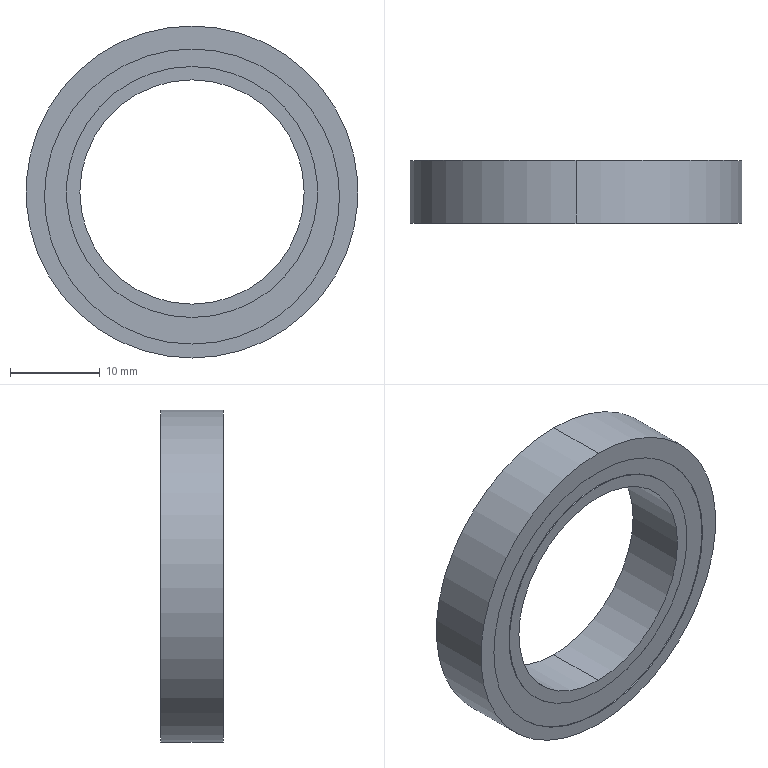Part | STEP file | Wheel bearing | 1 solid | 18 faces | box 37 x 7 x 37 mm | volume 4043 mm3 | cylinder 12 | plane 6 | commonest cylinder face diameters 27.974 x4 32.885 x4 25 x2 37 x2
STEP:
#1=CARTESIAN_POINT('',(0.,0.,0.));
#2=DIRECTION('',(0.,0.,1.));
#3=DIRECTION('',(1.,0.,0.));
#4=AXIS2_PLACEMENT_3D('',#1,#2,#3);
#5=CARTESIAN_POINT('',(0.,-3.4,13.987));
#6=VERTEX_POINT('',#5);
#7=CARTESIAN_POINT('',(0.,-3.4,-13.987));
#8=VERTEX_POINT('',#7);
#9=CARTESIAN_POINT('',(0.,-3.4,0.));
#10=DIRECTION('',(0.,1.,0.));
#11=DIRECTION('',(0.,0.,1.));
#12=AXIS2_PLACEMENT_3D('',#9,#10,#11);
#13=CIRCLE('',#12,13.987);
#14=CARTESIAN_POINT('',(0.,-3.4,0.));
#15=DIRECTION('',(0.,-1.,0.));
#16=DIRECTION('',(0.,0.,-1.));
#17=AXIS2_PLACEMENT_3D('',#14,#15,#16);
#18=CYLINDRICAL_SURFACE('',#17,13.987);
#19=CARTESIAN_POINT('',(3.142,0.));
#20=DIRECTION('',(-1.,0.));
#21=VECTOR('',#20,1.);
#22=LINE('',#19,#21);
#23=(GEOMETRIC_REPRESENTATION_CONTEXT(2)PARAMETRIC_REPRESENTATION_CONTEXT()REPRESENTATION_CONTEXT('',''));
#24=DEFINITIONAL_REPRESENTATION('',(#22),#23);
#25=PCURVE('',#18,#24);
#26=CARTESIAN_POINT('',(0.,-3.4,-0.506));
#27=DIRECTION('',(0.,-1.,0.));
#28=DIRECTION('',(0.,0.,1.));
#29=AXIS2_PLACEMENT_3D('',#26,#27,#28);
#30=PLANE('',#29);
#31=CARTESIAN_POINT('',(14.493,0.));
#32=CARTESIAN_POINT('',(14.493,-24.226));
#33=CARTESIAN_POINT('',(-6.487,-12.113));
#34=CARTESIAN_POINT('',(-27.468,0.));
#35=CARTESIAN_POINT('',(-6.487,12.113));
#36=CARTESIAN_POINT('',(14.493,24.226));
#37=CARTESIAN_POINT('',(14.493,0.));
#38=(BOUNDED_CURVE()B_SPLINE_CURVE(2,(#31,#32,#33,#34,#35,#36,#37),.UNSPECIFIED.,.T.,.F.)B_SPLINE_CURVE_WITH_KNOTS((1,2,2,2,2,1),(-2.094,0.,2.094,4.189,6.283,8.378),.UNSPECIFIED.)CURVE()GEOMETRIC_REPRESENTATION_ITEM()RATIONAL_B_SPLINE_CURVE((1.,0.5,1.,0.5,1.,0.5,1.))REPRESENTATION_ITEM(''));
#39=(GEOMETRIC_REPRESENTATION_CONTEXT(2)PARAMETRIC_REPRESENTATION_CONTEXT()REPRESENTATION_CONTEXT('',''));
#40=DEFINITIONAL_REPRESENTATION('',(#38),#39);
#41=PCURVE('',#30,#40);
#42=SURFACE_CURVE('',#13,(#25,#41),.PCURVE_S1.);
#43=EDGE_CURVE('',#6,#8,#42,.T.);
#44=ORIENTED_EDGE('',*,*,#43,.F.);
#45=CARTESIAN_POINT('',(0.,-3.5,13.987));
#46=VERTEX_POINT('',#45);
#47=CARTESIAN_POINT('',(0.,-3.4,13.987));
#48=DIRECTION('',(0.,-1.,0.));
#49=VECTOR('',#48,1.);
#50=LINE('',#47,#49);
#51=CARTESIAN_POINT('',(3.142,0.));
#52=DIRECTION('',(0.,1.));
#53=VECTOR('',#52,1.);
#54=LINE('',#51,#53);
#55=(GEOMETRIC_REPRESENTATION_CONTEXT(2)PARAMETRIC_REPRESENTATION_CONTEXT()REPRESENTATION_CONTEXT('',''));
#56=DEFINITIONAL_REPRESENTATION('',(#54),#55);
#57=PCURVE('',#18,#56);
#58=CARTESIAN_POINT('',(0.,-3.4,0.));
#59=DIRECTION('',(0.,-1.,0.));
#60=DIRECTION('',(0.,0.,-1.));
#61=AXIS2_PLACEMENT_3D('',#58,#59,#60);
#62=CYLINDRICAL_SURFACE('',#61,13.987);
#63=CARTESIAN_POINT('',(3.142,0.));
#64=DIRECTION('',(0.,1.));
#65=VECTOR('',#64,1.);
#66=LINE('',#63,#65);
#67=(GEOMETRIC_REPRESENTATION_CONTEXT(2)PARAMETRIC_REPRESENTATION_CONTEXT()REPRESENTATION_CONTEXT('',''));
#68=DEFINITIONAL_REPRESENTATION('',(#66),#67);
#69=PCURVE('',#62,#68);
#70=SURFACE_CURVE('',#50,(#57,#69),.PCURVE_S1.);
#71=EDGE_CURVE('',#6,#46,#70,.T.);
#72=ORIENTED_EDGE('',*,*,#71,.T.);
#73=CARTESIAN_POINT('',(0.,-3.5,-13.987));
#74=VERTEX_POINT('',#73);
#75=CARTESIAN_POINT('',(0.,-3.5,0.));
#76=DIRECTION('',(0.,1.,0.));
#77=DIRECTION('',(0.,0.,1.));
#78=AXIS2_PLACEMENT_3D('',#75,#76,#77);
#79=CIRCLE('',#78,13.987);
#80=CARTESIAN_POINT('',(3.142,0.1));
#81=DIRECTION('',(-1.,0.));
#82=VECTOR('',#81,1.);
#83=LINE('',#80,#82);
#84=(GEOMETRIC_REPRESENTATION_CONTEXT(2)PARAMETRIC_REPRESENTATION_CONTEXT()REPRESENTATION_CONTEXT('',''));
#85=DEFINITIONAL_REPRESENTATION('',(#83),#84);
#86=PCURVE('',#18,#85);
#87=CARTESIAN_POINT('',(0.,-3.5,0.));
#88=DIRECTION('',(0.,1.,0.));
#89=DIRECTION('',(0.,0.,1.));
#90=AXIS2_PLACEMENT_3D('',#87,#88,#89);
#91=PLANE('',#90);
#92=CARTESIAN_POINT('',(0.,0.));
#93=DIRECTION('',(1.,0.));
#94=AXIS2_PLACEMENT_2D('',#92,#93);
#95=CIRCLE('',#94,13.987);
#96=(GEOMETRIC_REPRESENTATION_CONTEXT(2)PARAMETRIC_REPRESENTATION_CONTEXT()REPRESENTATION_CONTEXT('',''));
#97=DEFINITIONAL_REPRESENTATION('',(#95),#96);
#98=PCURVE('',#91,#97);
#99=SURFACE_CURVE('',#79,(#86,#98),.PCURVE_S1.);
#100=EDGE_CURVE('',#46,#74,#99,.T.);
#101=ORIENTED_EDGE('',*,*,#100,.T.);
#102=CARTESIAN_POINT('',(0.,-3.4,-13.987));
#103=DIRECTION('',(0.,-1.,0.));
#104=VECTOR('',#103,1.);
#105=LINE('',#102,#104);
#106=CARTESIAN_POINT('',(0.,0.));
#107=DIRECTION('',(0.,1.));
#108=VECTOR('',#107,1.);
#109=LINE('',#106,#108);
#110=(GEOMETRIC_REPRESENTATION_CONTEXT(2)PARAMETRIC_REPRESENTATION_CONTEXT()REPRESENTATION_CONTEXT('',''));
#111=DEFINITIONAL_REPRESENTATION('',(#109),#110);
#112=PCURVE('',#18,#111);
#113=CARTESIAN_POINT('',(6.283,0.));
#114=DIRECTION('',(0.,1.));
#115=VECTOR('',#114,1.);
#116=LINE('',#113,#115);
#117=(GEOMETRIC_REPRESENTATION_CONTEXT(2)PARAMETRIC_REPRESENTATION_CONTEXT()REPRESENTATION_CONTEXT('',''));
#118=DEFINITIONAL_REPRESENTATION('',(#116),#117);
#119=PCURVE('',#62,#118);
#120=SURFACE_CURVE('',#105,(#112,#119),.PCURVE_S1.);
#121=EDGE_CURVE('',#8,#74,#120,.T.);
#122=ORIENTED_EDGE('',*,*,#121,.F.);
#123=EDGE_LOOP('',(#44,#72,#101,#122));
#124=FACE_BOUND('',#123,.T.);
#125=ADVANCED_FACE('',(#124),#18,.T.);
#126=CARTESIAN_POINT('',(0.,-3.4,-16.948));
#127=VERTEX_POINT('',#126);
#128=CARTESIAN_POINT('',(0.,-3.5,-16.948));
#129=VERTEX_POINT('',#128);
#130=CARTESIAN_POINT('',(0.,-3.4,-16.948));
#131=DIRECTION('',(0.,-1.,0.));
#132=VECTOR('',#131,1.);
#133=LINE('',#130,#132);
#134=CARTESIAN_POINT('',(0.,-3.4,-0.506));
#135=DIRECTION('',(0.,-1.,0.));
#136=DIRECTION('',(0.,0.,-1.));
#137=AXIS2_PLACEMENT_3D('',#134,#135,#136);
#138=CYLINDRICAL_SURFACE('',#137,16.442);
#139=CARTESIAN_POINT('',(6.283,0.));
#140=DIRECTION('',(0.,1.));
#141=VECTOR('',#140,1.);
#142=LINE('',#139,#141);
#143=(GEOMETRIC_REPRESENTATION_CONTEXT(2)PARAMETRIC_REPRESENTATION_CONTEXT()REPRESENTATION_CONTEXT('',''));
#144=DEFINITIONAL_REPRESENTATION('',(#142),#143);
#145=PCURVE('',#138,#144);
#146=CARTESIAN_POINT('',(0.,-3.4,-0.506));
#147=DIRECTION('',(0.,-1.,0.));
#148=DIRECTION('',(0.,0.,-1.));
#149=AXIS2_PLACEMENT_3D('',#146,#147,#148);
#150=CYLINDRICAL_SURFACE('',#149,16.442);
#151=CARTESIAN_POINT('',(0.,0.));
#152=DIRECTION('',(0.,1.));
#153=VECTOR('',#152,1.);
#154=LINE('',#151,#153);
#155=(GEOMETRIC_REPRESENTATION_CONTEXT(2)PARAMETRIC_REPRESENTATION_CONTEXT()REPRESENTATION_CONTEXT('',''));
#156=DEFINITIONAL_REPRESENTATION('',(#154),#155);
#157=PCURVE('',#150,#156);
#158=SURFACE_CURVE('',#133,(#145,#157),.PCURVE_S1.);
#159=EDGE_CURVE('',#127,#129,#158,.T.);
#160=ORIENTED_EDGE('',*,*,#159,.T.);
#161=CARTESIAN_POINT('',(0.,-3.5,15.936));
#162=VERTEX_POINT('',#161);
#163=CARTESIAN_POINT('',(0.,-3.5,-0.506));
#164=DIRECTION('',(0.,1.,0.));
#165=DIRECTION('',(0.,0.,1.));
#166=AXIS2_PLACEMENT_3D('',#163,#164,#165);
#167=CIRCLE('',#166,16.442);
#168=CARTESIAN_POINT('',(9.425,0.1));
#169=DIRECTION('',(-1.,0.));
#170=VECTOR('',#169,1.);
#171=LINE('',#168,#170);
#172=(GEOMETRIC_REPRESENTATION_CONTEXT(2)PARAMETRIC_REPRESENTATION_CONTEXT()REPRESENTATION_CONTEXT('',''));
#173=DEFINITIONAL_REPRESENTATION('',(#171),#172);
#174=PCURVE('',#138,#173);
#175=CARTESIAN_POINT('',(0.,-3.5,0.));
#176=DIRECTION('',(0.,1.,0.));
#177=DIRECTION('',(0.,0.,1.));
#178=AXIS2_PLACEMENT_3D('',#175,#176,#177);
#179=PLANE('',#178);
#180=CARTESIAN_POINT('',(-0.506,0.));
#181=DIRECTION('',(1.,0.));
#182=AXIS2_PLACEMENT_2D('',#180,#181);
#183=CIRCLE('',#182,16.442);
#184=(GEOMETRIC_REPRESENTATION_CONTEXT(2)PARAMETRIC_REPRESENTATION_CONTEXT()REPRESENTATION_CONTEXT('',''));
#185=DEFINITIONAL_REPRESENTATION('',(#183),#184);
#186=PCURVE('',#179,#185);
#187=SURFACE_CURVE('',#167,(#174,#186),.PCURVE_S1.);
#188=EDGE_CURVE('',#129,#162,#187,.T.);
#189=ORIENTED_EDGE('',*,*,#188,.T.);
#190=CARTESIAN_POINT('',(0.,-3.4,15.936));
#191=VERTEX_POINT('',#190);
#192=CARTESIAN_POINT('',(0.,-3.4,15.936));
#193=DIRECTION('',(0.,-1.,0.));
#194=VECTOR('',#193,1.);
#195=LINE('',#192,#194);
#196=CARTESIAN_POINT('',(3.142,0.));
#197=DIRECTION('',(0.,1.));
#198=VECTOR('',#197,1.);
#199=LINE('',#196,#198);
#200=(GEOMETRIC_REPRESENTATION_CONTEXT(2)PARAMETRIC_REPRESENTATION_CONTEXT()REPRESENTATION_CONTEXT('',''));
#201=DEFINITIONAL_REPRESENTATION('',(#199),#200);
#202=PCURVE('',#138,#201);
#203=CARTESIAN_POINT('',(3.142,0.));
#204=DIRECTION('',(0.,1.));
#205=VECTOR('',#204,1.);
#206=LINE('',#203,#205);
#207=(GEOMETRIC_REPRESENTATION_CONTEXT(2)PARAMETRIC_REPRESENTATION_CONTEXT()REPRESENTATION_CONTEXT('',''));
#208=DEFINITIONAL_REPRESENTATION('',(#206),#207);
#209=PCURVE('',#150,#208);
#210=SURFACE_CURVE('',#195,(#202,#209),.PCURVE_S1.);
#211=EDGE_CURVE('',#191,#162,#210,.T.);
#212=ORIENTED_EDGE('',*,*,#211,.F.);
#213=CARTESIAN_POINT('',(0.,-3.4,-0.506));
#214=DIRECTION('',(0.,1.,0.));
#215=DIRECTION('',(0.,0.,1.));
#216=AXIS2_PLACEMENT_3D('',#213,#214,#215);
#217=CIRCLE('',#216,16.442);
#218=CARTESIAN_POINT('',(9.425,0.));
#219=DIRECTION('',(-1.,0.));
#220=VECTOR('',#219,1.);
#221=LINE('',#218,#220);
#222=(GEOMETRIC_REPRESENTATION_CONTEXT(2)PARAMETRIC_REPRESENTATION_CONTEXT()REPRESENTATION_CONTEXT('',''));
#223=DEFINITIONAL_REPRESENTATION('',(#221),#222);
#224=PCURVE('',#138,#223);
#225=CARTESIAN_POINT('',(16.442,0.));
#226=CARTESIAN_POINT('',(16.442,-28.479));
#227=CARTESIAN_POINT('',(-8.221,-14.239));
#228=CARTESIAN_POINT('',(-32.885,0.));
#229=CARTESIAN_POINT('',(-8.221,14.239));
#230=CARTESIAN_POINT('',(16.442,28.479));
#231=CARTESIAN_POINT('',(16.442,0.));
#232=(BOUNDED_CURVE()B_SPLINE_CURVE(2,(#225,#226,#227,#228,#229,#230,#231),.UNSPECIFIED.,.T.,.F.)B_SPLINE_CURVE_WITH_KNOTS((1,2,2,2,2,1),(-2.094,0.,2.094,4.189,6.283,8.378),.UNSPECIFIED.)CURVE()GEOMETRIC_REPRESENTATION_ITEM()RATIONAL_B_SPLINE_CURVE((1.,0.5,1.,0.5,1.,0.5,1.))REPRESENTATION_ITEM(''));
#233=(GEOMETRIC_REPRESENTATION_CONTEXT(2)PARAMETRIC_REPRESENTATION_CONTEXT()REPRESENTATION_CONTEXT('',''));
#234=DEFINITIONAL_REPRESENTATION('',(#232),#233);
#235=PCURVE('',#30,#234);
#236=SURFACE_CURVE('',#217,(#224,#235),.PCURVE_S1.);
#237=EDGE_CURVE('',#127,#191,#236,.T.);
#238=ORIENTED_EDGE('',*,*,#237,.F.);
#239=EDGE_LOOP('',(#160,#189,#212,#238));
#240=FACE_BOUND('',#239,.F.);
#241=ADVANCED_FACE('',(#240),#138,.F.);
#242=CARTESIAN_POINT('',(0.,3.4,13.987));
#243=VERTEX_POINT('',#242);
#244=CARTESIAN_POINT('',(0.,3.4,-13.987));
#245=VERTEX_POINT('',#244);
#246=CARTESIAN_POINT('',(0.,3.4,0.));
#247=DIRECTION('',(0.,1.,0.));
#248=DIRECTION('',(0.,0.,1.));
#249=AXIS2_PLACEMENT_3D('',#246,#247,#248);
#250=CIRCLE('',#249,13.987);
#251=CARTESIAN_POINT('',(0.,3.4,0.));
#252=DIRECTION('',(0.,1.,0.));
#253=DIRECTION('',(0.,0.,1.));
#254=AXIS2_PLACEMENT_3D('',#251,#252,#253);
#255=CYLINDRICAL_SURFACE('',#254,13.987);
#256=CARTESIAN_POINT('',(0.,0.));
#257=DIRECTION('',(1.,0.));
#258=VECTOR('',#257,1.);
#259=LINE('',#256,#258);
#260=(GEOMETRIC_REPRESENTATION_CONTEXT(2)PARAMETRIC_REPRESENTATION_CONTEXT()REPRESENTATION_CONTEXT('',''));
#261=DEFINITIONAL_REPRESENTATION('',(#259),#260);
#262=PCURVE('',#255,#261);
#263=CARTESIAN_POINT('',(0.,3.4,-0.506));
#264=DIRECTION('',(0.,1.,0.));
#265=DIRECTION('',(0.,0.,1.));
#266=AXIS2_PLACEMENT_3D('',#263,#264,#265);
#267=PLANE('',#266);
#268=CARTESIAN_POINT('',(0.506,0.));
#269=DIRECTION('',(1.,0.));
#270=AXIS2_PLACEMENT_2D('',#268,#269);
#271=CIRCLE('',#270,13.987);
#272=(GEOMETRIC_REPRESENTATION_CONTEXT(2)PARAMETRIC_REPRESENTATION_CONTEXT()REPRESENTATION_CONTEXT('',''));
#273=DEFINITIONAL_REPRESENTATION('',(#271),#272);
#274=PCURVE('',#267,#273);
#275=SURFACE_CURVE('',#250,(#262,#274),.PCURVE_S1.);
#276=EDGE_CURVE('',#243,#245,#275,.T.);
#277=ORIENTED_EDGE('',*,*,#276,.T.);
#278=CARTESIAN_POINT('',(0.,3.5,-13.987));
#279=VERTEX_POINT('',#278);
#280=CARTESIAN_POINT('',(0.,3.4,-13.987));
#281=DIRECTION('',(0.,1.,0.));
#282=VECTOR('',#281,1.);
#283=LINE('',#280,#282);
#284=CARTESIAN_POINT('',(3.142,0.));
#285=DIRECTION('',(0.,1.));
#286=VECTOR('',#285,1.);
#287=LINE('',#284,#286);
#288=(GEOMETRIC_REPRESENTATION_CONTEXT(2)PARAMETRIC_REPRESENTATION_CONTEXT()REPRESENTATION_CONTEXT('',''));
#289=DEFINITIONAL_REPRESENTATION('',(#287),#288);
#290=PCURVE('',#255,#289);
#291=CARTESIAN_POINT('',(0.,3.4,0.));
#292=DIRECTION('',(0.,1.,0.));
#293=DIRECTION('',(0.,0.,1.));
#294=AXIS2_PLACEMENT_3D('',#291,#292,#293);
#295=CYLINDRICAL_SURFACE('',#294,13.987);
#296=CARTESIAN_POINT('',(3.142,0.));
#297=DIRECTION('',(0.,1.));
#298=VECTOR('',#297,1.);
#299=LINE('',#296,#298);
#300=(GEOMETRIC_REPRESENTATION_CONTEXT(2)PARAMETRIC_REPRESENTATION_CONTEXT()REPRESENTATION_CONTEXT('',''));
#301=DEFINITIONAL_REPRESENTATION('',(#299),#300);
#302=PCURVE('',#295,#301);
#303=SURFACE_CURVE('',#283,(#290,#302),.PCURVE_S1.);
#304=EDGE_CURVE('',#245,#279,#303,.T.);
#305=ORIENTED_EDGE('',*,*,#304,.T.);
#306=CARTESIAN_POINT('',(0.,3.5,13.987));
#307=VERTEX_POINT('',#306);
#308=CARTESIAN_POINT('',(0.,3.5,0.));
#309=DIRECTION('',(0.,1.,0.));
#310=DIRECTION('',(0.,0.,1.));
#311=AXIS2_PLACEMENT_3D('',#308,#309,#310);
#312=CIRCLE('',#311,13.987);
#313=CARTESIAN_POINT('',(0.,0.1));
#314=DIRECTION('',(1.,0.));
#315=VECTOR('',#314,1.);
#316=LINE('',#313,#315);
#317=(GEOMETRIC_REPRESENTATION_CONTEXT(2)PARAMETRIC_REPRESENTATION_CONTEXT()REPRESENTATION_CONTEXT('',''));
#318=DEFINITIONAL_REPRESENTATION('',(#316),#317);
#319=PCURVE('',#255,#318);
#320=CARTESIAN_POINT('',(0.,3.5,0.));
#321=DIRECTION('',(0.,1.,0.));
#322=DIRECTION('',(0.,0.,1.));
#323=AXIS2_PLACEMENT_3D('',#320,#321,#322);
#324=PLANE('',#323);
#325=CARTESIAN_POINT('',(0.,0.));
#326=DIRECTION('',(1.,0.));
#327=AXIS2_PLACEMENT_2D('',#325,#326);
#328=CIRCLE('',#327,13.987);
#329=(GEOMETRIC_REPRESENTATION_CONTEXT(2)PARAMETRIC_REPRESENTATION_CONTEXT()REPRESENTATION_CONTEXT('',''));
#330=DEFINITIONAL_REPRESENTATION('',(#328),#329);
#331=PCURVE('',#324,#330);
#332=SURFACE_CURVE('',#312,(#319,#331),.PCURVE_S1.);
#333=EDGE_CURVE('',#307,#279,#332,.T.);
#334=ORIENTED_EDGE('',*,*,#333,.F.);
#335=CARTESIAN_POINT('',(0.,3.4,13.987));
#336=DIRECTION('',(0.,1.,0.));
#337=VECTOR('',#336,1.);
#338=LINE('',#335,#337);
#339=CARTESIAN_POINT('',(0.,0.));
#340=DIRECTION('',(0.,1.));
#341=VECTOR('',#340,1.);
#342=LINE('',#339,#341);
#343=(GEOMETRIC_REPRESENTATION_CONTEXT(2)PARAMETRIC_REPRESENTATION_CONTEXT()REPRESENTATION_CONTEXT('',''));
#344=DEFINITIONAL_REPRESENTATION('',(#342),#343);
#345=PCURVE('',#255,#344);
#346=CARTESIAN_POINT('',(6.283,0.));
#347=DIRECTION('',(0.,1.));
#348=VECTOR('',#347,1.);
#349=LINE('',#346,#348);
#350=(GEOMETRIC_REPRESENTATION_CONTEXT(2)PARAMETRIC_REPRESENTATION_CONTEXT()REPRESENTATION_CONTEXT('',''));
#351=DEFINITIONAL_REPRESENTATION('',(#349),#350);
#352=PCURVE('',#295,#351);
#353=SURFACE_CURVE('',#338,(#345,#352),.PCURVE_S1.);
#354=EDGE_CURVE('',#243,#307,#353,.T.);
#355=ORIENTED_EDGE('',*,*,#354,.F.);
#356=EDGE_LOOP('',(#277,#305,#334,#355));
#357=FACE_BOUND('',#356,.T.);
#358=ADVANCED_FACE('',(#357),#255,.T.);
#359=CARTESIAN_POINT('',(0.,3.4,15.936));
#360=VERTEX_POINT('',#359);
#361=CARTESIAN_POINT('',(0.,3.5,15.936));
#362=VERTEX_POINT('',#361);
#363=CARTESIAN_POINT('',(0.,3.4,15.936));
#364=DIRECTION('',(0.,1.,0.));
#365=VECTOR('',#364,1.);
#366=LINE('',#363,#365);
#367=CARTESIAN_POINT('',(0.,3.4,-0.506));
#368=DIRECTION('',(0.,1.,0.));
#369=DIRECTION('',(0.,0.,1.));
#370=AXIS2_PLACEMENT_3D('',#367,#368,#369);
#371=CYLINDRICAL_SURFACE('',#370,16.442);
#372=CARTESIAN_POINT('',(6.283,0.));
#373=DIRECTION('',(0.,1.));
#374=VECTOR('',#373,1.);
#375=LINE('',#372,#374);
#376=(GEOMETRIC_REPRESENTATION_CONTEXT(2)PARAMETRIC_REPRESENTATION_CONTEXT()REPRESENTATION_CONTEXT('',''));
#377=DEFINITIONAL_REPRESENTATION('',(#375),#376);
#378=PCURVE('',#371,#377);
#379=CARTESIAN_POINT('',(0.,3.4,-0.506));
#380=DIRECTION('',(0.,1.,0.));
#381=DIRECTION('',(0.,0.,1.));
#382=AXIS2_PLACEMENT_3D('',#379,#380,#381);
#383=CYLINDRICAL_SURFACE('',#382,16.442);
#384=CARTESIAN_POINT('',(0.,0.));
#385=DIRECTION('',(0.,1.));
#386=VECTOR('',#385,1.);
#387=LINE('',#384,#386);
#388=(GEOMETRIC_REPRESENTATION_CONTEXT(2)PARAMETRIC_REPRESENTATION_CONTEXT()REPRESENTATION_CONTEXT('',''));
#389=DEFINITIONAL_REPRESENTATION('',(#387),#388);
#390=PCURVE('',#383,#389);
#391=SURFACE_CURVE('',#366,(#378,#390),.PCURVE_S1.);
#392=EDGE_CURVE('',#360,#362,#391,.T.);
#393=ORIENTED_EDGE('',*,*,#392,.T.);
#394=CARTESIAN_POINT('',(0.,3.5,-16.948));
#395=VERTEX_POINT('',#394);
#396=CARTESIAN_POINT('',(0.,3.5,-0.506));
#397=DIRECTION('',(0.,1.,0.));
#398=DIRECTION('',(0.,0.,1.));
#399=AXIS2_PLACEMENT_3D('',#396,#397,#398);
#400=CIRCLE('',#399,16.442);
#401=CARTESIAN_POINT('',(0.,0.1));
#402=DIRECTION('',(1.,0.));
#403=VECTOR('',#402,1.);
#404=LINE('',#401,#403);
#405=(GEOMETRIC_REPRESENTATION_CONTEXT(2)PARAMETRIC_REPRESENTATION_CONTEXT()REPRESENTATION_CONTEXT('',''));
#406=DEFINITIONAL_REPRESENTATION('',(#404),#405);
#407=PCURVE('',#371,#406);
#408=CARTESIAN_POINT('',(0.,3.5,0.));
#409=DIRECTION('',(0.,1.,0.));
#410=DIRECTION('',(0.,0.,1.));
#411=AXIS2_PLACEMENT_3D('',#408,#409,#410);
#412=PLANE('',#411);
#413=CARTESIAN_POINT('',(-0.506,0.));
#414=DIRECTION('',(1.,0.));
#415=AXIS2_PLACEMENT_2D('',#413,#414);
#416=CIRCLE('',#415,16.442);
#417=(GEOMETRIC_REPRESENTATION_CONTEXT(2)PARAMETRIC_REPRESENTATION_CONTEXT()REPRESENTATION_CONTEXT('',''));
#418=DEFINITIONAL_REPRESENTATION('',(#416),#417);
#419=PCURVE('',#412,#418);
#420=SURFACE_CURVE('',#400,(#407,#419),.PCURVE_S1.);
#421=EDGE_CURVE('',#395,#362,#420,.T.);
#422=ORIENTED_EDGE('',*,*,#421,.F.);
#423=CARTESIAN_POINT('',(0.,3.4,-16.948));
#424=VERTEX_POINT('',#423);
#425=CARTESIAN_POINT('',(0.,3.4,-16.948));
#426=DIRECTION('',(0.,1.,0.));
#427=VECTOR('',#426,1.);
#428=LINE('',#425,#427);
#429=CARTESIAN_POINT('',(3.142,0.));
#430=DIRECTION('',(0.,1.));
#431=VECTOR('',#430,1.);
#432=LINE('',#429,#431);
#433=(GEOMETRIC_REPRESENTATION_CONTEXT(2)PARAMETRIC_REPRESENTATION_CONTEXT()REPRESENTATION_CONTEXT('',''));
#434=DEFINITIONAL_REPRESENTATION('',(#432),#433);
#435=PCURVE('',#371,#434);
#436=CARTESIAN_POINT('',(3.142,0.));
#437=DIRECTION('',(0.,1.));
#438=VECTOR('',#437,1.);
#439=LINE('',#436,#438);
#440=(GEOMETRIC_REPRESENTATION_CONTEXT(2)PARAMETRIC_REPRESENTATION_CONTEXT()REPRESENTATION_CONTEXT('',''));
#441=DEFINITIONAL_REPRESENTATION('',(#439),#440);
#442=PCURVE('',#383,#441);
#443=SURFACE_CURVE('',#428,(#435,#442),.PCURVE_S1.);
#444=EDGE_CURVE('',#424,#395,#443,.T.);
#445=ORIENTED_EDGE('',*,*,#444,.F.);
#446=CARTESIAN_POINT('',(0.,3.4,-0.506));
#447=DIRECTION('',(0.,1.,0.));
#448=DIRECTION('',(0.,0.,1.));
#449=AXIS2_PLACEMENT_3D('',#446,#447,#448);
#450=CIRCLE('',#449,16.442);
#451=CARTESIAN_POINT('',(0.,0.));
#452=DIRECTION('',(1.,0.));
#453=VECTOR('',#452,1.);
#454=LINE('',#451,#453);
#455=(GEOMETRIC_REPRESENTATION_CONTEXT(2)PARAMETRIC_REPRESENTATION_CONTEXT()REPRESENTATION_CONTEXT('',''));
#456=DEFINITIONAL_REPRESENTATION('',(#454),#455);
#457=PCURVE('',#371,#456);
#458=CARTESIAN_POINT('',(0.,0.));
#459=DIRECTION('',(1.,0.));
#460=AXIS2_PLACEMENT_2D('',#458,#459);
#461=CIRCLE('',#460,16.442);
#462=(GEOMETRIC_REPRESENTATION_CONTEXT(2)PARAMETRIC_REPRESENTATION_CONTEXT()REPRESENTATION_CONTEXT('',''));
#463=DEFINITIONAL_REPRESENTATION('',(#461),#462);
#464=PCURVE('',#267,#463);
#465=SURFACE_CURVE('',#450,(#457,#464),.PCURVE_S1.);
#466=EDGE_CURVE('',#424,#360,#465,.T.);
#467=ORIENTED_EDGE('',*,*,#466,.T.);
#468=EDGE_LOOP('',(#393,#422,#445,#467));
#469=FACE_BOUND('',#468,.F.);
#470=ADVANCED_FACE('',(#469),#371,.F.);
#471=CARTESIAN_POINT('',(0.,3.5,-12.5));
#472=VERTEX_POINT('',#471);
#473=CARTESIAN_POINT('',(0.,-3.5,-12.5));
#474=VERTEX_POINT('',#473);
#475=CARTESIAN_POINT('',(0.,3.5,-12.5));
#476=DIRECTION('',(0.,-1.,0.));
#477=VECTOR('',#476,1.);
#478=LINE('',#475,#477);
#479=CARTESIAN_POINT('',(0.,3.5,0.));
#480=DIRECTION('',(0.,-1.,0.));
#481=DIRECTION('',(0.,0.,-1.));
#482=AXIS2_PLACEMENT_3D('',#479,#480,#481);
#483=CYLINDRICAL_SURFACE('',#482,12.5);
#484=CARTESIAN_POINT('',(6.283,0.));
#485=DIRECTION('',(0.,1.));
#486=VECTOR('',#485,1.);
#487=LINE('',#484,#486);
#488=(GEOMETRIC_REPRESENTATION_CONTEXT(2)PARAMETRIC_REPRESENTATION_CONTEXT()REPRESENTATION_CONTEXT('',''));
#489=DEFINITIONAL_REPRESENTATION('',(#487),#488);
#490=PCURVE('',#483,#489);
#491=CARTESIAN_POINT('',(0.,3.5,0.));
#492=DIRECTION('',(0.,-1.,0.));
#493=DIRECTION('',(0.,0.,-1.));
#494=AXIS2_PLACEMENT_3D('',#491,#492,#493);
#495=CYLINDRICAL_SURFACE('',#494,12.5);
#496=CARTESIAN_POINT('',(0.,0.));
#497=DIRECTION('',(0.,1.));
#498=VECTOR('',#497,1.);
#499=LINE('',#496,#498);
#500=(GEOMETRIC_REPRESENTATION_CONTEXT(2)PARAMETRIC_REPRESENTATION_CONTEXT()REPRESENTATION_CONTEXT('',''));
#501=DEFINITIONAL_REPRESENTATION('',(#499),#500);
#502=PCURVE('',#495,#501);
#503=SURFACE_CURVE('',#478,(#490,#502),.PCURVE_S1.);
#504=EDGE_CURVE('',#472,#474,#503,.T.);
#505=ORIENTED_EDGE('',*,*,#504,.T.);
#506=CARTESIAN_POINT('',(0.,-3.5,12.5));
#507=VERTEX_POINT('',#506);
#508=CARTESIAN_POINT('',(0.,-3.5,0.));
#509=DIRECTION('',(0.,1.,0.));
#510=DIRECTION('',(0.,0.,1.));
#511=AXIS2_PLACEMENT_3D('',#508,#509,#510);
#512=CIRCLE('',#511,12.5);
#513=CARTESIAN_POINT('',(9.425,7.));
#514=DIRECTION('',(-1.,0.));
#515=VECTOR('',#514,1.);
#516=LINE('',#513,#515);
#517=(GEOMETRIC_REPRESENTATION_CONTEXT(2)PARAMETRIC_REPRESENTATION_CONTEXT()REPRESENTATION_CONTEXT('',''));
#518=DEFINITIONAL_REPRESENTATION('',(#516),#517);
#519=PCURVE('',#483,#518);
#520=CARTESIAN_POINT('',(0.,0.));
#521=DIRECTION('',(1.,0.));
#522=AXIS2_PLACEMENT_2D('',#520,#521);
#523=CIRCLE('',#522,12.5);
#524=(GEOMETRIC_REPRESENTATION_CONTEXT(2)PARAMETRIC_REPRESENTATION_CONTEXT()REPRESENTATION_CONTEXT('',''));
#525=DEFINITIONAL_REPRESENTATION('',(#523),#524);
#526=PCURVE('',#91,#525);
#527=SURFACE_CURVE('',#512,(#519,#526),.PCURVE_S1.);
#528=EDGE_CURVE('',#474,#507,#527,.T.);
#529=ORIENTED_EDGE('',*,*,#528,.T.);
#530=CARTESIAN_POINT('',(0.,3.5,12.5));
#531=VERTEX_POINT('',#530);
#532=CARTESIAN_POINT('',(0.,3.5,12.5));
#533=DIRECTION('',(0.,-1.,0.));
#534=VECTOR('',#533,1.);
#535=LINE('',#532,#534);
#536=CARTESIAN_POINT('',(3.142,0.));
#537=DIRECTION('',(0.,1.));
#538=VECTOR('',#537,1.);
#539=LINE('',#536,#538);
#540=(GEOMETRIC_REPRESENTATION_CONTEXT(2)PARAMETRIC_REPRESENTATION_CONTEXT()REPRESENTATION_CONTEXT('',''));
#541=DEFINITIONAL_REPRESENTATION('',(#539),#540);
#542=PCURVE('',#483,#541);
#543=CARTESIAN_POINT('',(3.142,0.));
#544=DIRECTION('',(0.,1.));
#545=VECTOR('',#544,1.);
#546=LINE('',#543,#545);
#547=(GEOMETRIC_REPRESENTATION_CONTEXT(2)PARAMETRIC_REPRESENTATION_CONTEXT()REPRESENTATION_CONTEXT('',''));
#548=DEFINITIONAL_REPRESENTATION('',(#546),#547);
#549=PCURVE('',#495,#548);
#550=SURFACE_CURVE('',#535,(#542,#549),.PCURVE_S1.);
#551=EDGE_CURVE('',#531,#507,#550,.T.);
#552=ORIENTED_EDGE('',*,*,#551,.F.);
#553=CARTESIAN_POINT('',(0.,3.5,0.));
#554=DIRECTION('',(0.,1.,0.));
#555=DIRECTION('',(0.,0.,1.));
#556=AXIS2_PLACEMENT_3D('',#553,#554,#555);
#557=CIRCLE('',#556,12.5);
#558=CARTESIAN_POINT('',(9.425,0.));
#559=DIRECTION('',(-1.,0.));
#560=VECTOR('',#559,1.);
#561=LINE('',#558,#560);
#562=(GEOMETRIC_REPRESENTATION_CONTEXT(2)PARAMETRIC_REPRESENTATION_CONTEXT()REPRESENTATION_CONTEXT('',''));
#563=DEFINITIONAL_REPRESENTATION('',(#561),#562);
#564=PCURVE('',#483,#563);
#565=CARTESIAN_POINT('',(0.,0.));
#566=DIRECTION('',(1.,0.));
#567=AXIS2_PLACEMENT_2D('',#565,#566);
#568=CIRCLE('',#567,12.5);
#569=(GEOMETRIC_REPRESENTATION_CONTEXT(2)PARAMETRIC_REPRESENTATION_CONTEXT()REPRESENTATION_CONTEXT('',''));
#570=DEFINITIONAL_REPRESENTATION('',(#568),#569);
#571=PCURVE('',#324,#570);
#572=SURFACE_CURVE('',#557,(#564,#571),.PCURVE_S1.);
#573=EDGE_CURVE('',#472,#531,#572,.T.);
#574=ORIENTED_EDGE('',*,*,#573,.F.);
#575=EDGE_LOOP('',(#505,#529,#552,#574));
#576=FACE_BOUND('',#575,.F.);
#577=ADVANCED_FACE('',(#576),#483,.F.);
#578=CARTESIAN_POINT('',(0.,3.5,18.5));
#579=VERTEX_POINT('',#578);
#580=CARTESIAN_POINT('',(0.,3.5,-18.5));
#581=VERTEX_POINT('',#580);
#582=CARTESIAN_POINT('',(0.,3.5,0.));
#583=DIRECTION('',(0.,1.,0.));
#584=DIRECTION('',(0.,0.,1.));
#585=AXIS2_PLACEMENT_3D('',#582,#583,#584);
#586=CIRCLE('',#585,18.5);
#587=CARTESIAN_POINT('',(0.,3.5,0.));
#588=DIRECTION('',(0.,-1.,0.));
#589=DIRECTION('',(0.,0.,-1.));
#590=AXIS2_PLACEMENT_3D('',#587,#588,#589);
#591=CYLINDRICAL_SURFACE('',#590,18.5);
#592=CARTESIAN_POINT('',(3.142,0.));
#593=DIRECTION('',(-1.,0.));
#594=VECTOR('',#593,1.);
#595=LINE('',#592,#594);
#596=(GEOMETRIC_REPRESENTATION_CONTEXT(2)PARAMETRIC_REPRESENTATION_CONTEXT()REPRESENTATION_CONTEXT('',''));
#597=DEFINITIONAL_REPRESENTATION('',(#595),#596);
#598=PCURVE('',#591,#597);
#599=CARTESIAN_POINT('',(0.,0.));
#600=DIRECTION('',(1.,0.));
#601=AXIS2_PLACEMENT_2D('',#599,#600);
#602=CIRCLE('',#601,18.5);
#603=(GEOMETRIC_REPRESENTATION_CONTEXT(2)PARAMETRIC_REPRESENTATION_CONTEXT()REPRESENTATION_CONTEXT('',''));
#604=DEFINITIONAL_REPRESENTATION('',(#602),#603);
#605=PCURVE('',#412,#604);
#606=SURFACE_CURVE('',#586,(#598,#605),.PCURVE_S1.);
#607=EDGE_CURVE('',#579,#581,#606,.T.);
#608=ORIENTED_EDGE('',*,*,#607,.F.);
#609=CARTESIAN_POINT('',(0.,-3.5,18.5));
#610=VERTEX_POINT('',#609);
#611=CARTESIAN_POINT('',(0.,3.5,18.5));
#612=DIRECTION('',(0.,-1.,0.));
#613=VECTOR('',#612,1.);
#614=LINE('',#611,#613);
#615=CARTESIAN_POINT('',(3.142,0.));
#616=DIRECTION('',(0.,1.));
#617=VECTOR('',#616,1.);
#618=LINE('',#615,#617);
#619=(GEOMETRIC_REPRESENTATION_CONTEXT(2)PARAMETRIC_REPRESENTATION_CONTEXT()REPRESENTATION_CONTEXT('',''));
#620=DEFINITIONAL_REPRESENTATION('',(#618),#619);
#621=PCURVE('',#591,#620);
#622=CARTESIAN_POINT('',(0.,3.5,0.));
#623=DIRECTION('',(0.,-1.,0.));
#624=DIRECTION('',(0.,0.,-1.));
#625=AXIS2_PLACEMENT_3D('',#622,#623,#624);
#626=CYLINDRICAL_SURFACE('',#625,18.5);
#627=CARTESIAN_POINT('',(3.142,0.));
#628=DIRECTION('',(0.,1.));
#629=VECTOR('',#628,1.);
#630=LINE('',#627,#629);
#631=(GEOMETRIC_REPRESENTATION_CONTEXT(2)PARAMETRIC_REPRESENTATION_CONTEXT()REPRESENTATION_CONTEXT('',''));
#632=DEFINITIONAL_REPRESENTATION('',(#630),#631);
#633=PCURVE('',#626,#632);
#634=SURFACE_CURVE('',#614,(#621,#633),.PCURVE_S1.);
#635=EDGE_CURVE('',#579,#610,#634,.T.);
#636=ORIENTED_EDGE('',*,*,#635,.T.);
#637=CARTESIAN_POINT('',(0.,-3.5,-18.5));
#638=VERTEX_POINT('',#637);
#639=CARTESIAN_POINT('',(0.,-3.5,0.));
#640=DIRECTION('',(0.,1.,0.));
#641=DIRECTION('',(0.,0.,1.));
#642=AXIS2_PLACEMENT_3D('',#639,#640,#641);
#643=CIRCLE('',#642,18.5);
#644=CARTESIAN_POINT('',(3.142,7.));
#645=DIRECTION('',(-1.,0.));
#646=VECTOR('',#645,1.);
#647=LINE('',#644,#646);
#648=(GEOMETRIC_REPRESENTATION_CONTEXT(2)PARAMETRIC_REPRESENTATION_CONTEXT()REPRESENTATION_CONTEXT('',''));
#649=DEFINITIONAL_REPRESENTATION('',(#647),#648);
#650=PCURVE('',#591,#649);
#651=CARTESIAN_POINT('',(0.,0.));
#652=DIRECTION('',(1.,0.));
#653=AXIS2_PLACEMENT_2D('',#651,#652);
#654=CIRCLE('',#653,18.5);
#655=(GEOMETRIC_REPRESENTATION_CONTEXT(2)PARAMETRIC_REPRESENTATION_CONTEXT()REPRESENTATION_CONTEXT('',''));
#656=DEFINITIONAL_REPRESENTATION('',(#654),#655);
#657=PCURVE('',#179,#656);
#658=SURFACE_CURVE('',#643,(#650,#657),.PCURVE_S1.);
#659=EDGE_CURVE('',#610,#638,#658,.T.);
#660=ORIENTED_EDGE('',*,*,#659,.T.);
#661=CARTESIAN_POINT('',(0.,3.5,-18.5));
#662=DIRECTION('',(0.,-1.,0.));
#663=VECTOR('',#662,1.);
#664=LINE('',#661,#663);
#665=CARTESIAN_POINT('',(0.,0.));
#666=DIRECTION('',(0.,1.));
#667=VECTOR('',#666,1.);
#668=LINE('',#665,#667);
#669=(GEOMETRIC_REPRESENTATION_CONTEXT(2)PARAMETRIC_REPRESENTATION_CONTEXT()REPRESENTATION_CONTEXT('',''));
#670=DEFINITIONAL_REPRESENTATION('',(#668),#669);
#671=PCURVE('',#591,#670);
#672=CARTESIAN_POINT('',(6.283,0.));
#673=DIRECTION('',(0.,1.));
#674=VECTOR('',#673,1.);
#675=LINE('',#672,#674);
#676=(GEOMETRIC_REPRESENTATION_CONTEXT(2)PARAMETRIC_REPRESENTATION_CONTEXT()REPRESENTATION_CONTEXT('',''));
#677=DEFINITIONAL_REPRESENTATION('',(#675),#676);
#678=PCURVE('',#626,#677);
#679=SURFACE_CURVE('',#664,(#671,#678),.PCURVE_S1.);
#680=EDGE_CURVE('',#581,#638,#679,.T.);
#681=ORIENTED_EDGE('',*,*,#680,.F.);
#682=EDGE_LOOP('',(#608,#636,#660,#681));
#683=FACE_BOUND('',#682,.T.);
#684=ADVANCED_FACE('',(#683),#591,.T.);
#685=ORIENTED_EDGE('',*,*,#528,.T.);
#686=CARTESIAN_POINT('',(0.,-3.5,0.));
#687=DIRECTION('',(0.,1.,0.));
#688=DIRECTION('',(0.,0.,1.));
#689=AXIS2_PLACEMENT_3D('',#686,#687,#688);
#690=CIRCLE('',#689,12.5);
#691=CARTESIAN_POINT('',(0.,0.));
#692=DIRECTION('',(1.,0.));
#693=AXIS2_PLACEMENT_2D('',#691,#692);
#694=CIRCLE('',#693,12.5);
#695=(GEOMETRIC_REPRESENTATION_CONTEXT(2)PARAMETRIC_REPRESENTATION_CONTEXT()REPRESENTATION_CONTEXT('',''));
#696=DEFINITIONAL_REPRESENTATION('',(#694),#695);
#697=PCURVE('',#91,#696);
#698=CARTESIAN_POINT('',(3.142,7.));
#699=DIRECTION('',(-1.,0.));
#700=VECTOR('',#699,1.);
#701=LINE('',#698,#700);
#702=(GEOMETRIC_REPRESENTATION_CONTEXT(2)PARAMETRIC_REPRESENTATION_CONTEXT()REPRESENTATION_CONTEXT('',''));
#703=DEFINITIONAL_REPRESENTATION('',(#701),#702);
#704=PCURVE('',#495,#703);
#705=SURFACE_CURVE('',#690,(#697,#704),.PCURVE_S1.);
#706=EDGE_CURVE('',#507,#474,#705,.T.);
#707=ORIENTED_EDGE('',*,*,#706,.T.);
#708=EDGE_LOOP('',(#685,#707));
#709=FACE_BOUND('',#708,.T.);
#710=CARTESIAN_POINT('',(0.,-3.5,0.));
#711=DIRECTION('',(0.,1.,0.));
#712=DIRECTION('',(0.,0.,1.));
#713=AXIS2_PLACEMENT_3D('',#710,#711,#712);
#714=CIRCLE('',#713,13.987);
#715=CARTESIAN_POINT('',(0.,0.));
#716=DIRECTION('',(1.,0.));
#717=AXIS2_PLACEMENT_2D('',#715,#716);
#718=CIRCLE('',#717,13.987);
#719=(GEOMETRIC_REPRESENTATION_CONTEXT(2)PARAMETRIC_REPRESENTATION_CONTEXT()REPRESENTATION_CONTEXT('',''));
#720=DEFINITIONAL_REPRESENTATION('',(#718),#719);
#721=PCURVE('',#91,#720);
#722=CARTESIAN_POINT('',(9.425,0.1));
#723=DIRECTION('',(-1.,0.));
#724=VECTOR('',#723,1.);
#725=LINE('',#722,#724);
#726=(GEOMETRIC_REPRESENTATION_CONTEXT(2)PARAMETRIC_REPRESENTATION_CONTEXT()REPRESENTATION_CONTEXT('',''));
#727=DEFINITIONAL_REPRESENTATION('',(#725),#726);
#728=PCURVE('',#62,#727);
#729=SURFACE_CURVE('',#714,(#721,#728),.PCURVE_S1.);
#730=EDGE_CURVE('',#74,#46,#729,.T.);
#731=ORIENTED_EDGE('',*,*,#730,.F.);
#732=ORIENTED_EDGE('',*,*,#100,.F.);
#733=EDGE_LOOP('',(#731,#732));
#734=FACE_BOUND('',#733,.T.);
#735=ADVANCED_FACE('',(#709,#734),#91,.F.);
#736=ORIENTED_EDGE('',*,*,#573,.F.);
#737=CARTESIAN_POINT('',(0.,3.5,0.));
#738=DIRECTION('',(0.,1.,0.));
#739=DIRECTION('',(0.,0.,1.));
#740=AXIS2_PLACEMENT_3D('',#737,#738,#739);
#741=CIRCLE('',#740,12.5);
#742=CARTESIAN_POINT('',(0.,0.));
#743=DIRECTION('',(1.,0.));
#744=AXIS2_PLACEMENT_2D('',#742,#743);
#745=CIRCLE('',#744,12.5);
#746=(GEOMETRIC_REPRESENTATION_CONTEXT(2)PARAMETRIC_REPRESENTATION_CONTEXT()REPRESENTATION_CONTEXT('',''));
#747=DEFINITIONAL_REPRESENTATION('',(#745),#746);
#748=PCURVE('',#324,#747);
#749=CARTESIAN_POINT('',(3.142,0.));
#750=DIRECTION('',(-1.,0.));
#751=VECTOR('',#750,1.);
#752=LINE('',#749,#751);
#753=(GEOMETRIC_REPRESENTATION_CONTEXT(2)PARAMETRIC_REPRESENTATION_CONTEXT()REPRESENTATION_CONTEXT('',''));
#754=DEFINITIONAL_REPRESENTATION('',(#752),#753);
#755=PCURVE('',#495,#754);
#756=SURFACE_CURVE('',#741,(#748,#755),.PCURVE_S1.);
#757=EDGE_CURVE('',#531,#472,#756,.T.);
#758=ORIENTED_EDGE('',*,*,#757,.F.);
#759=EDGE_LOOP('',(#736,#758));
#760=FACE_BOUND('',#759,.T.);
#761=ORIENTED_EDGE('',*,*,#333,.T.);
#762=CARTESIAN_POINT('',(0.,3.5,0.));
#763=DIRECTION('',(0.,1.,0.));
#764=DIRECTION('',(0.,0.,1.));
#765=AXIS2_PLACEMENT_3D('',#762,#763,#764);
#766=CIRCLE('',#765,13.987);
#767=CARTESIAN_POINT('',(0.,0.));
#768=DIRECTION('',(1.,0.));
#769=AXIS2_PLACEMENT_2D('',#767,#768);
#770=CIRCLE('',#769,13.987);
#771=(GEOMETRIC_REPRESENTATION_CONTEXT(2)PARAMETRIC_REPRESENTATION_CONTEXT()REPRESENTATION_CONTEXT('',''));
#772=DEFINITIONAL_REPRESENTATION('',(#770),#771);
#773=PCURVE('',#324,#772);
#774=CARTESIAN_POINT('',(0.,0.1));
#775=DIRECTION('',(1.,0.));
#776=VECTOR('',#775,1.);
#777=LINE('',#774,#776);
#778=(GEOMETRIC_REPRESENTATION_CONTEXT(2)PARAMETRIC_REPRESENTATION_CONTEXT()REPRESENTATION_CONTEXT('',''));
#779=DEFINITIONAL_REPRESENTATION('',(#777),#778);
#780=PCURVE('',#295,#779);
#781=SURFACE_CURVE('',#766,(#773,#780),.PCURVE_S1.);
#782=EDGE_CURVE('',#279,#307,#781,.T.);
#783=ORIENTED_EDGE('',*,*,#782,.T.);
#784=EDGE_LOOP('',(#761,#783));
#785=FACE_BOUND('',#784,.T.);
#786=ADVANCED_FACE('',(#760,#785),#324,.T.);
#787=CARTESIAN_POINT('',(0.,3.5,-0.506));
#788=DIRECTION('',(0.,1.,0.));
#789=DIRECTION('',(0.,0.,1.));
#790=AXIS2_PLACEMENT_3D('',#787,#788,#789);
#791=CIRCLE('',#790,16.442);
#792=CARTESIAN_POINT('',(-0.506,0.));
#793=DIRECTION('',(1.,0.));
#794=AXIS2_PLACEMENT_2D('',#792,#793);
#795=CIRCLE('',#794,16.442);
#796=(GEOMETRIC_REPRESENTATION_CONTEXT(2)PARAMETRIC_REPRESENTATION_CONTEXT()REPRESENTATION_CONTEXT('',''));
#797=DEFINITIONAL_REPRESENTATION('',(#795),#796);
#798=PCURVE('',#412,#797);
#799=CARTESIAN_POINT('',(0.,0.1));
#800=DIRECTION('',(1.,0.));
#801=VECTOR('',#800,1.);
#802=LINE('',#799,#801);
#803=(GEOMETRIC_REPRESENTATION_CONTEXT(2)PARAMETRIC_REPRESENTATION_CONTEXT()REPRESENTATION_CONTEXT('',''));
#804=DEFINITIONAL_REPRESENTATION('',(#802),#803);
#805=PCURVE('',#383,#804);
#806=SURFACE_CURVE('',#791,(#798,#805),.PCURVE_S1.);
#807=EDGE_CURVE('',#362,#395,#806,.T.);
#808=ORIENTED_EDGE('',*,*,#807,.F.);
#809=ORIENTED_EDGE('',*,*,#421,.F.);
#810=EDGE_LOOP('',(#808,#809));
#811=FACE_BOUND('',#810,.T.);
#812=CARTESIAN_POINT('',(0.,3.5,0.));
#813=DIRECTION('',(0.,1.,0.));
#814=DIRECTION('',(0.,0.,1.));
#815=AXIS2_PLACEMENT_3D('',#812,#813,#814);
#816=CIRCLE('',#815,18.5);
#817=CARTESIAN_POINT('',(0.,0.));
#818=DIRECTION('',(1.,0.));
#819=AXIS2_PLACEMENT_2D('',#817,#818);
#820=CIRCLE('',#819,18.5);
#821=(GEOMETRIC_REPRESENTATION_CONTEXT(2)PARAMETRIC_REPRESENTATION_CONTEXT()REPRESENTATION_CONTEXT('',''));
#822=DEFINITIONAL_REPRESENTATION('',(#820),#821);
#823=PCURVE('',#412,#822);
#824=CARTESIAN_POINT('',(9.425,0.));
#825=DIRECTION('',(-1.,0.));
#826=VECTOR('',#825,1.);
#827=LINE('',#824,#826);
#828=(GEOMETRIC_REPRESENTATION_CONTEXT(2)PARAMETRIC_REPRESENTATION_CONTEXT()REPRESENTATION_CONTEXT('',''));
#829=DEFINITIONAL_REPRESENTATION('',(#827),#828);
#830=PCURVE('',#626,#829);
#831=SURFACE_CURVE('',#816,(#823,#830),.PCURVE_S1.);
#832=EDGE_CURVE('',#581,#579,#831,.T.);
#833=ORIENTED_EDGE('',*,*,#832,.T.);
#834=ORIENTED_EDGE('',*,*,#607,.T.);
#835=EDGE_LOOP('',(#833,#834));
#836=FACE_BOUND('',#835,.T.);
#837=ADVANCED_FACE('',(#811,#836),#412,.T.);
#838=ORIENTED_EDGE('',*,*,#188,.T.);
#839=CARTESIAN_POINT('',(0.,-3.5,-0.506));
#840=DIRECTION('',(0.,1.,0.));
#841=DIRECTION('',(0.,0.,1.));
#842=AXIS2_PLACEMENT_3D('',#839,#840,#841);
#843=CIRCLE('',#842,16.442);
#844=CARTESIAN_POINT('',(-0.506,0.));
#845=DIRECTION('',(1.,0.));
#846=AXIS2_PLACEMENT_2D('',#844,#845);
#847=CIRCLE('',#846,16.442);
#848=(GEOMETRIC_REPRESENTATION_CONTEXT(2)PARAMETRIC_REPRESENTATION_CONTEXT()REPRESENTATION_CONTEXT('',''));
#849=DEFINITIONAL_REPRESENTATION('',(#847),#848);
#850=PCURVE('',#179,#849);
#851=CARTESIAN_POINT('',(3.142,0.1));
#852=DIRECTION('',(-1.,0.));
#853=VECTOR('',#852,1.);
#854=LINE('',#851,#853);
#855=(GEOMETRIC_REPRESENTATION_CONTEXT(2)PARAMETRIC_REPRESENTATION_CONTEXT()REPRESENTATION_CONTEXT('',''));
#856=DEFINITIONAL_REPRESENTATION('',(#854),#855);
#857=PCURVE('',#150,#856);
#858=SURFACE_CURVE('',#843,(#850,#857),.PCURVE_S1.);
#859=EDGE_CURVE('',#162,#129,#858,.T.);
#860=ORIENTED_EDGE('',*,*,#859,.T.);
#861=EDGE_LOOP('',(#838,#860));
#862=FACE_BOUND('',#861,.T.);
#863=CARTESIAN_POINT('',(0.,-3.5,0.));
#864=DIRECTION('',(0.,1.,0.));
#865=DIRECTION('',(0.,0.,1.));
#866=AXIS2_PLACEMENT_3D('',#863,#864,#865);
#867=CIRCLE('',#866,18.5);
#868=CARTESIAN_POINT('',(0.,0.));
#869=DIRECTION('',(1.,0.));
#870=AXIS2_PLACEMENT_2D('',#868,#869);
#871=CIRCLE('',#870,18.5);
#872=(GEOMETRIC_REPRESENTATION_CONTEXT(2)PARAMETRIC_REPRESENTATION_CONTEXT()REPRESENTATION_CONTEXT('',''));
#873=DEFINITIONAL_REPRESENTATION('',(#871),#872);
#874=PCURVE('',#179,#873);
#875=CARTESIAN_POINT('',(9.425,7.));
#876=DIRECTION('',(-1.,0.));
#877=VECTOR('',#876,1.);
#878=LINE('',#875,#877);
#879=(GEOMETRIC_REPRESENTATION_CONTEXT(2)PARAMETRIC_REPRESENTATION_CONTEXT()REPRESENTATION_CONTEXT('',''));
#880=DEFINITIONAL_REPRESENTATION('',(#878),#879);
#881=PCURVE('',#626,#880);
#882=SURFACE_CURVE('',#867,(#874,#881),.PCURVE_S1.);
#883=EDGE_CURVE('',#638,#610,#882,.T.);
#884=ORIENTED_EDGE('',*,*,#883,.F.);
#885=ORIENTED_EDGE('',*,*,#659,.F.);
#886=EDGE_LOOP('',(#884,#885));
#887=FACE_BOUND('',#886,.T.);
#888=ADVANCED_FACE('',(#862,#887),#179,.F.);
#889=ORIENTED_EDGE('',*,*,#635,.F.);
#890=ORIENTED_EDGE('',*,*,#832,.F.);
#891=ORIENTED_EDGE('',*,*,#680,.T.);
#892=ORIENTED_EDGE('',*,*,#883,.T.);
#893=EDGE_LOOP('',(#889,#890,#891,#892));
#894=FACE_BOUND('',#893,.T.);
#895=ADVANCED_FACE('',(#894),#626,.T.);
#896=ORIENTED_EDGE('',*,*,#706,.T.);
#897=ORIENTED_EDGE('',*,*,#504,.F.);
#898=ORIENTED_EDGE('',*,*,#757,.F.);
#899=ORIENTED_EDGE('',*,*,#551,.T.);
#900=EDGE_LOOP('',(#896,#897,#898,#899));
#901=FACE_BOUND('',#900,.F.);
#902=ADVANCED_FACE('',(#901),#495,.F.);
#903=ORIENTED_EDGE('',*,*,#807,.F.);
#904=ORIENTED_EDGE('',*,*,#392,.F.);
#905=CARTESIAN_POINT('',(0.,3.4,-0.506));
#906=DIRECTION('',(0.,1.,0.));
#907=DIRECTION('',(0.,0.,1.));
#908=AXIS2_PLACEMENT_3D('',#905,#906,#907);
#909=CIRCLE('',#908,16.442);
#910=CARTESIAN_POINT('',(0.,0.));
#911=DIRECTION('',(1.,0.));
#912=VECTOR('',#911,1.);
#913=LINE('',#910,#912);
#914=(GEOMETRIC_REPRESENTATION_CONTEXT(2)PARAMETRIC_REPRESENTATION_CONTEXT()REPRESENTATION_CONTEXT('',''));
#915=DEFINITIONAL_REPRESENTATION('',(#913),#914);
#916=PCURVE('',#383,#915);
#917=CARTESIAN_POINT('',(0.,0.));
#918=DIRECTION('',(1.,0.));
#919=AXIS2_PLACEMENT_2D('',#917,#918);
#920=CIRCLE('',#919,16.442);
#921=(GEOMETRIC_REPRESENTATION_CONTEXT(2)PARAMETRIC_REPRESENTATION_CONTEXT()REPRESENTATION_CONTEXT('',''));
#922=DEFINITIONAL_REPRESENTATION('',(#920),#921);
#923=PCURVE('',#267,#922);
#924=SURFACE_CURVE('',#909,(#916,#923),.PCURVE_S1.);
#925=EDGE_CURVE('',#360,#424,#924,.T.);
#926=ORIENTED_EDGE('',*,*,#925,.T.);
#927=ORIENTED_EDGE('',*,*,#444,.T.);
#928=EDGE_LOOP('',(#903,#904,#926,#927));
#929=FACE_BOUND('',#928,.F.);
#930=ADVANCED_FACE('',(#929),#383,.F.);
#931=ORIENTED_EDGE('',*,*,#276,.F.);
#932=CARTESIAN_POINT('',(0.,3.4,0.));
#933=DIRECTION('',(0.,1.,0.));
#934=DIRECTION('',(0.,0.,1.));
#935=AXIS2_PLACEMENT_3D('',#932,#933,#934);
#936=CIRCLE('',#935,13.987);
#937=CARTESIAN_POINT('',(0.506,0.));
#938=DIRECTION('',(1.,0.));
#939=AXIS2_PLACEMENT_2D('',#937,#938);
#940=CIRCLE('',#939,13.987);
#941=(GEOMETRIC_REPRESENTATION_CONTEXT(2)PARAMETRIC_REPRESENTATION_CONTEXT()REPRESENTATION_CONTEXT('',''));
#942=DEFINITIONAL_REPRESENTATION('',(#940),#941);
#943=PCURVE('',#267,#942);
#944=CARTESIAN_POINT('',(0.,0.));
#945=DIRECTION('',(1.,0.));
#946=VECTOR('',#945,1.);
#947=LINE('',#944,#946);
#948=(GEOMETRIC_REPRESENTATION_CONTEXT(2)PARAMETRIC_REPRESENTATION_CONTEXT()REPRESENTATION_CONTEXT('',''));
#949=DEFINITIONAL_REPRESENTATION('',(#947),#948);
#950=PCURVE('',#295,#949);
#951=SURFACE_CURVE('',#936,(#943,#950),.PCURVE_S1.);
#952=EDGE_CURVE('',#245,#243,#951,.T.);
#953=ORIENTED_EDGE('',*,*,#952,.F.);
#954=EDGE_LOOP('',(#931,#953));
#955=FACE_BOUND('',#954,.T.);
#956=ORIENTED_EDGE('',*,*,#925,.T.);
#957=ORIENTED_EDGE('',*,*,#466,.T.);
#958=EDGE_LOOP('',(#956,#957));
#959=FACE_BOUND('',#958,.T.);
#960=ADVANCED_FACE('',(#955,#959),#267,.T.);
#961=ORIENTED_EDGE('',*,*,#304,.F.);
#962=ORIENTED_EDGE('',*,*,#952,.T.);
#963=ORIENTED_EDGE('',*,*,#354,.T.);
#964=ORIENTED_EDGE('',*,*,#782,.F.);
#965=EDGE_LOOP('',(#961,#962,#963,#964));
#966=FACE_BOUND('',#965,.T.);
#967=ADVANCED_FACE('',(#966),#295,.T.);
#968=ORIENTED_EDGE('',*,*,#237,.F.);
#969=CARTESIAN_POINT('',(0.,-3.4,-0.506));
#970=DIRECTION('',(0.,1.,0.));
#971=DIRECTION('',(0.,0.,1.));
#972=AXIS2_PLACEMENT_3D('',#969,#970,#971);
#973=CIRCLE('',#972,16.442);
#974=CARTESIAN_POINT('',(16.442,0.));
#975=CARTESIAN_POINT('',(16.442,-28.479));
#976=CARTESIAN_POINT('',(-8.221,-14.239));
#977=CARTESIAN_POINT('',(-32.885,0.));
#978=CARTESIAN_POINT('',(-8.221,14.239));
#979=CARTESIAN_POINT('',(16.442,28.479));
#980=CARTESIAN_POINT('',(16.442,0.));
#981=(BOUNDED_CURVE()B_SPLINE_CURVE(2,(#974,#975,#976,#977,#978,#979,#980),.UNSPECIFIED.,.T.,.F.)B_SPLINE_CURVE_WITH_KNOTS((1,2,2,2,2,1),(-2.094,0.,2.094,4.189,6.283,8.378),.UNSPECIFIED.)CURVE()GEOMETRIC_REPRESENTATION_ITEM()RATIONAL_B_SPLINE_CURVE((1.,0.5,1.,0.5,1.,0.5,1.))REPRESENTATION_ITEM(''));
#982=(GEOMETRIC_REPRESENTATION_CONTEXT(2)PARAMETRIC_REPRESENTATION_CONTEXT()REPRESENTATION_CONTEXT('',''));
#983=DEFINITIONAL_REPRESENTATION('',(#981),#982);
#984=PCURVE('',#30,#983);
#985=CARTESIAN_POINT('',(3.142,0.));
#986=DIRECTION('',(-1.,0.));
#987=VECTOR('',#986,1.);
#988=LINE('',#985,#987);
#989=(GEOMETRIC_REPRESENTATION_CONTEXT(2)PARAMETRIC_REPRESENTATION_CONTEXT()REPRESENTATION_CONTEXT('',''));
#990=DEFINITIONAL_REPRESENTATION('',(#988),#989);
#991=PCURVE('',#150,#990);
#992=SURFACE_CURVE('',#973,(#984,#991),.PCURVE_S1.);
#993=EDGE_CURVE('',#191,#127,#992,.T.);
#994=ORIENTED_EDGE('',*,*,#993,.F.);
#995=EDGE_LOOP('',(#968,#994));
#996=FACE_BOUND('',#995,.T.);
#997=CARTESIAN_POINT('',(0.,-3.4,0.));
#998=DIRECTION('',(0.,1.,0.));
#999=DIRECTION('',(0.,0.,1.));
#1000=AXIS2_PLACEMENT_3D('',#997,#998,#999);
#1001=CIRCLE('',#1000,13.987);
#1002=CARTESIAN_POINT('',(14.493,0.));
#1003=CARTESIAN_POINT('',(14.493,-24.226));
#1004=CARTESIAN_POINT('',(-6.487,-12.113));
#1005=CARTESIAN_POINT('',(-27.468,0.));
#1006=CARTESIAN_POINT('',(-6.487,12.113));
#1007=CARTESIAN_POINT('',(14.493,24.226));
#1008=CARTESIAN_POINT('',(14.493,0.));
#1009=(BOUNDED_CURVE()B_SPLINE_CURVE(2,(#1002,#1003,#1004,#1005,#1006,#1007,#1008),.UNSPECIFIED.,.T.,.F.)B_SPLINE_CURVE_WITH_KNOTS((1,2,2,2,2,1),(-2.094,0.,2.094,4.189,6.283,8.378),.UNSPECIFIED.)CURVE()GEOMETRIC_REPRESENTATION_ITEM()RATIONAL_B_SPLINE_CURVE((1.,0.5,1.,0.5,1.,0.5,1.))REPRESENTATION_ITEM(''));
#1010=(GEOMETRIC_REPRESENTATION_CONTEXT(2)PARAMETRIC_REPRESENTATION_CONTEXT()REPRESENTATION_CONTEXT('',''));
#1011=DEFINITIONAL_REPRESENTATION('',(#1009),#1010);
#1012=PCURVE('',#30,#1011);
#1013=CARTESIAN_POINT('',(9.425,0.));
#1014=DIRECTION('',(-1.,0.));
#1015=VECTOR('',#1014,1.);
#1016=LINE('',#1013,#1015);
#1017=(GEOMETRIC_REPRESENTATION_CONTEXT(2)PARAMETRIC_REPRESENTATION_CONTEXT()REPRESENTATION_CONTEXT('',''));
#1018=DEFINITIONAL_REPRESENTATION('',(#1016),#1017);
#1019=PCURVE('',#62,#1018);
#1020=SURFACE_CURVE('',#1001,(#1012,#1019),.PCURVE_S1.);
#1021=EDGE_CURVE('',#8,#6,#1020,.T.);
#1022=ORIENTED_EDGE('',*,*,#1021,.T.);
#1023=ORIENTED_EDGE('',*,*,#43,.T.);
#1024=EDGE_LOOP('',(#1022,#1023));
#1025=FACE_BOUND('',#1024,.T.);
#1026=ADVANCED_FACE('',(#996,#1025),#30,.T.);
#1027=ORIENTED_EDGE('',*,*,#859,.T.);
#1028=ORIENTED_EDGE('',*,*,#159,.F.);
#1029=ORIENTED_EDGE('',*,*,#993,.F.);
#1030=ORIENTED_EDGE('',*,*,#211,.T.);
#1031=EDGE_LOOP('',(#1027,#1028,#1029,#1030));
#1032=FACE_BOUND('',#1031,.F.);
#1033=ADVANCED_FACE('',(#1032),#150,.F.);
#1034=ORIENTED_EDGE('',*,*,#71,.F.);
#1035=ORIENTED_EDGE('',*,*,#1021,.F.);
#1036=ORIENTED_EDGE('',*,*,#121,.T.);
#1037=ORIENTED_EDGE('',*,*,#730,.T.);
#1038=EDGE_LOOP('',(#1034,#1035,#1036,#1037));
#1039=FACE_BOUND('',#1038,.T.);
#1040=ADVANCED_FACE('',(#1039),#62,.T.);
#1041=CLOSED_SHELL('',(#125,#241,#358,#470,#577,#684,#735,#786,#837,#888,#895,#902,#930,#960,#967,#1026,#1033,#1040));
#1042=MANIFOLD_SOLID_BREP('',#1041);
#1043=(LENGTH_UNIT()NAMED_UNIT(*)SI_UNIT(.MILLI.,.METRE.));
#1044=UNCERTAINTY_MEASURE_WITH_UNIT(LENGTH_MEASURE(0.0000001),#1043,'','');
#1045=(NAMED_UNIT(*)PLANE_ANGLE_UNIT()SI_UNIT($,.RADIAN.));
#1046=(NAMED_UNIT(*)SI_UNIT($,.STERADIAN.)SOLID_ANGLE_UNIT());
#1047=(GEOMETRIC_REPRESENTATION_CONTEXT(3)GLOBAL_UNCERTAINTY_ASSIGNED_CONTEXT((#1044))GLOBAL_UNIT_ASSIGNED_CONTEXT((#1043,#1045,#1046))REPRESENTATION_CONTEXT('',''));
#1048=ADVANCED_BREP_SHAPE_REPRESENTATION('',(#4,#1042),#1047);